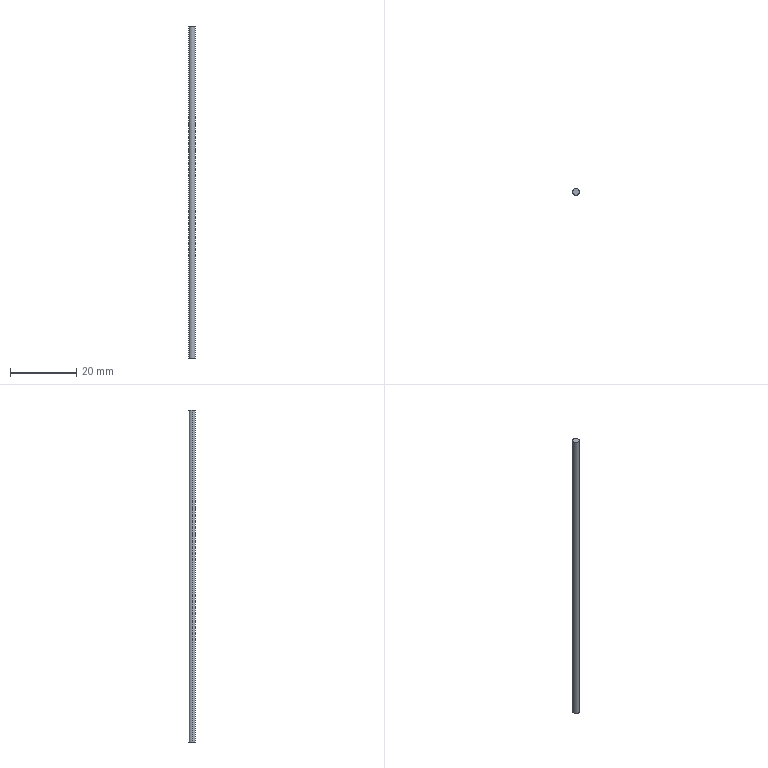Part | STEP file | 102000006984 | 1 solid | 4 faces | box 2 x 2 x 100 mm | volume 314.159 mm3 | cylinder 2 | plane 2 | commonest cylinder face diameters 2 x2
STEP:
#1=CARTESIAN_POINT('',(1.,0.,100.));
#2=VERTEX_POINT('',#1);
#3=CARTESIAN_POINT('',(-1.,0.,100.));
#4=VERTEX_POINT('',#3);
#5=CARTESIAN_POINT('',(0.,0.,100.));
#6=DIRECTION('',(0.,0.,-1.));
#7=AXIS2_PLACEMENT_3D('',#5,#6,$);
#8=CIRCLE('',#7,1.);
#9=EDGE_CURVE('',#2,#4,#8,.F.);
#10=ORIENTED_EDGE('',*,*,#9,.F.);
#11=CARTESIAN_POINT('',(1.,0.,0.));
#12=VERTEX_POINT('',#11);
#13=CARTESIAN_POINT('',(1.,0.,100.));
#14=DIRECTION('',(0.,0.,-1.));
#15=VECTOR('',#14,1.);
#16=LINE('',#13,#15);
#17=EDGE_CURVE('',#2,#12,#16,.T.);
#18=ORIENTED_EDGE('',*,*,#17,.T.);
#19=CARTESIAN_POINT('',(-1.,0.,0.));
#20=VERTEX_POINT('',#19);
#21=CARTESIAN_POINT('',(0.,0.,0.));
#22=DIRECTION('',(0.,0.,-1.));
#23=AXIS2_PLACEMENT_3D('',#21,#22,$);
#24=CIRCLE('',#23,1.);
#25=EDGE_CURVE('',#12,#20,#24,.F.);
#26=ORIENTED_EDGE('',*,*,#25,.T.);
#27=CARTESIAN_POINT('',(-1.,0.,100.));
#28=DIRECTION('',(0.,0.,-1.));
#29=VECTOR('',#28,1.);
#30=LINE('',#27,#29);
#31=EDGE_CURVE('',#4,#20,#30,.T.);
#32=ORIENTED_EDGE('',*,*,#31,.F.);
#33=EDGE_LOOP('',(#10,#18,#26,#32));
#34=FACE_OUTER_BOUND('',#33,.T.);
#35=CARTESIAN_POINT('',(0.,0.,100.));
#36=DIRECTION('',(0.,0.,-1.));
#37=DIRECTION('',(-1.,0.,0.));
#38=AXIS2_PLACEMENT_3D('',#35,#36,#37);
#39=CYLINDRICAL_SURFACE('',#38,1.);
#40=ADVANCED_FACE('',(#34),#39,.T.);
#41=CARTESIAN_POINT('',(0.,0.,100.));
#42=DIRECTION('',(0.,0.,1.));
#43=AXIS2_PLACEMENT_3D('',#41,#42,$);
#44=CIRCLE('',#43,1.);
#45=EDGE_CURVE('',#4,#2,#44,.T.);
#46=ORIENTED_EDGE('',*,*,#45,.T.);
#47=ORIENTED_EDGE('',*,*,#9,.T.);
#48=EDGE_LOOP('',(#46,#47));
#49=FACE_OUTER_BOUND('',#48,.T.);
#50=CARTESIAN_POINT('',(0.,0.,100.));
#51=DIRECTION('',(0.,0.,1.));
#52=DIRECTION('',(1.,0.,0.));
#53=AXIS2_PLACEMENT_3D('',#50,#51,#52);
#54=PLANE('',#53);
#55=ADVANCED_FACE('',(#49),#54,.T.);
#56=ORIENTED_EDGE('',*,*,#17,.F.);
#57=ORIENTED_EDGE('',*,*,#45,.F.);
#58=ORIENTED_EDGE('',*,*,#31,.T.);
#59=CARTESIAN_POINT('',(0.,0.,0.));
#60=DIRECTION('',(0.,0.,-1.));
#61=AXIS2_PLACEMENT_3D('',#59,#60,$);
#62=CIRCLE('',#61,1.);
#63=EDGE_CURVE('',#20,#12,#62,.F.);
#64=ORIENTED_EDGE('',*,*,#63,.T.);
#65=EDGE_LOOP('',(#56,#57,#58,#64));
#66=FACE_OUTER_BOUND('',#65,.T.);
#67=CARTESIAN_POINT('',(0.,0.,100.));
#68=DIRECTION('',(0.,0.,-1.));
#69=DIRECTION('',(1.,0.,0.));
#70=AXIS2_PLACEMENT_3D('',#67,#68,#69);
#71=CYLINDRICAL_SURFACE('',#70,1.);
#72=ADVANCED_FACE('',(#66),#71,.T.);
#73=ORIENTED_EDGE('',*,*,#63,.F.);
#74=ORIENTED_EDGE('',*,*,#25,.F.);
#75=EDGE_LOOP('',(#73,#74));
#76=FACE_OUTER_BOUND('',#75,.T.);
#77=CARTESIAN_POINT('',(0.,0.,0.));
#78=DIRECTION('',(0.,0.,1.));
#79=DIRECTION('',(1.,0.,0.));
#80=AXIS2_PLACEMENT_3D('',#77,#78,#79);
#81=PLANE('',#80);
#82=ADVANCED_FACE('',(#76),#81,.F.);
#83=CLOSED_SHELL('',(#40,#55,#72,#82));
#84=MANIFOLD_SOLID_BREP('',#83);
#85=(LENGTH_UNIT()NAMED_UNIT(*)SI_UNIT(.MILLI.,.METRE.));
#86=UNCERTAINTY_MEASURE_WITH_UNIT(LENGTH_MEASURE(0.005),#85,'','');
#87=(NAMED_UNIT(*)PLANE_ANGLE_UNIT()SI_UNIT($,.RADIAN.));
#88=(NAMED_UNIT(*)SI_UNIT($,.STERADIAN.)SOLID_ANGLE_UNIT());
#89=(GEOMETRIC_REPRESENTATION_CONTEXT(3)GLOBAL_UNCERTAINTY_ASSIGNED_CONTEXT((#86))GLOBAL_UNIT_ASSIGNED_CONTEXT((#85,#87,#88))REPRESENTATION_CONTEXT('',''));
#90=ADVANCED_BREP_SHAPE_REPRESENTATION('',(#84),#89);